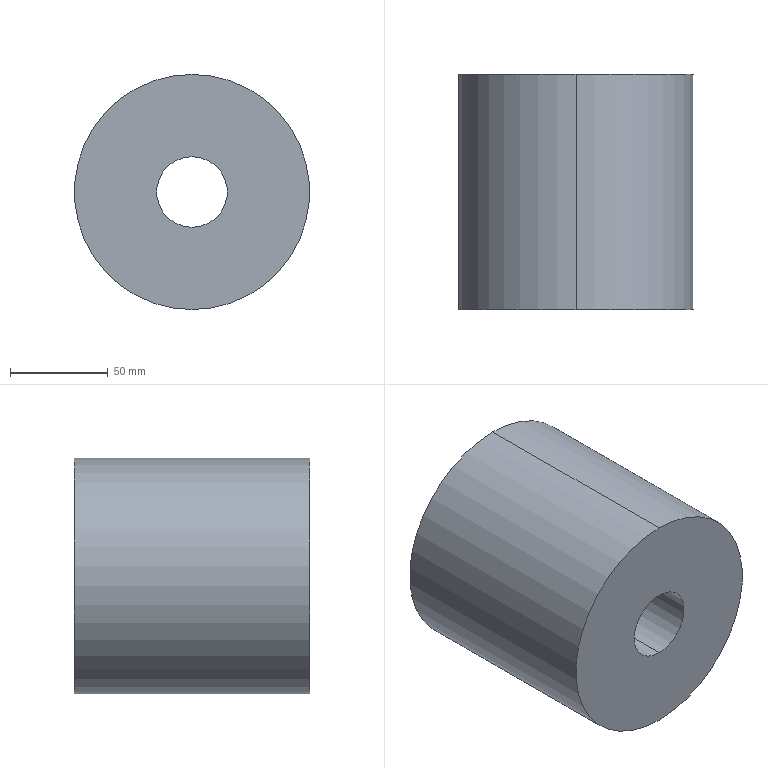Part | STEP file | 1 solid | 6 faces | box 120 x 120 x 120 mm | volume 1235023 mm3 | cylinder 4 | plane 2 | commonest cylinder face diameters 36 x2 120 x2
STEP:
#1=CARTESIAN_POINT('',(0.,0.,0.));
#2=DIRECTION('',(0.,0.,1.));
#3=DIRECTION('',(1.,0.,0.));
#4=AXIS2_PLACEMENT_3D('',#1,#2,#3);
#5=CARTESIAN_POINT('',(0.,60.,-18.));
#6=VERTEX_POINT('',#5);
#7=CARTESIAN_POINT('',(0.,-60.,-18.));
#8=VERTEX_POINT('',#7);
#9=CARTESIAN_POINT('',(0.,60.,-18.));
#10=DIRECTION('',(0.,-1.,0.));
#11=VECTOR('',#10,1.);
#12=LINE('',#9,#11);
#13=CARTESIAN_POINT('',(0.,60.,0.));
#14=DIRECTION('',(0.,-1.,0.));
#15=DIRECTION('',(0.,0.,-1.));
#16=AXIS2_PLACEMENT_3D('',#13,#14,#15);
#17=CYLINDRICAL_SURFACE('',#16,18.);
#18=CARTESIAN_POINT('',(6.283,0.));
#19=DIRECTION('',(0.,1.));
#20=VECTOR('',#19,1.);
#21=LINE('',#18,#20);
#22=(GEOMETRIC_REPRESENTATION_CONTEXT(2)PARAMETRIC_REPRESENTATION_CONTEXT()REPRESENTATION_CONTEXT('',''));
#23=DEFINITIONAL_REPRESENTATION('',(#21),#22);
#24=PCURVE('',#17,#23);
#25=CARTESIAN_POINT('',(0.,60.,0.));
#26=DIRECTION('',(0.,-1.,0.));
#27=DIRECTION('',(0.,0.,-1.));
#28=AXIS2_PLACEMENT_3D('',#25,#26,#27);
#29=CYLINDRICAL_SURFACE('',#28,18.);
#30=CARTESIAN_POINT('',(0.,0.));
#31=DIRECTION('',(0.,1.));
#32=VECTOR('',#31,1.);
#33=LINE('',#30,#32);
#34=(GEOMETRIC_REPRESENTATION_CONTEXT(2)PARAMETRIC_REPRESENTATION_CONTEXT()REPRESENTATION_CONTEXT('',''));
#35=DEFINITIONAL_REPRESENTATION('',(#33),#34);
#36=PCURVE('',#29,#35);
#37=SURFACE_CURVE('',#12,(#24,#36),.PCURVE_S1.);
#38=EDGE_CURVE('',#6,#8,#37,.T.);
#39=ORIENTED_EDGE('',*,*,#38,.T.);
#40=CARTESIAN_POINT('',(0.,-60.,18.));
#41=VERTEX_POINT('',#40);
#42=CARTESIAN_POINT('',(0.,-60.,0.));
#43=DIRECTION('',(0.,1.,0.));
#44=DIRECTION('',(0.,0.,1.));
#45=AXIS2_PLACEMENT_3D('',#42,#43,#44);
#46=CIRCLE('',#45,18.);
#47=CARTESIAN_POINT('',(9.425,120.));
#48=DIRECTION('',(-1.,0.));
#49=VECTOR('',#48,1.);
#50=LINE('',#47,#49);
#51=(GEOMETRIC_REPRESENTATION_CONTEXT(2)PARAMETRIC_REPRESENTATION_CONTEXT()REPRESENTATION_CONTEXT('',''));
#52=DEFINITIONAL_REPRESENTATION('',(#50),#51);
#53=PCURVE('',#17,#52);
#54=CARTESIAN_POINT('',(0.,-60.,0.));
#55=DIRECTION('',(0.,1.,0.));
#56=DIRECTION('',(0.,0.,1.));
#57=AXIS2_PLACEMENT_3D('',#54,#55,#56);
#58=PLANE('',#57);
#59=CARTESIAN_POINT('',(0.,0.));
#60=DIRECTION('',(1.,0.));
#61=AXIS2_PLACEMENT_2D('',#59,#60);
#62=CIRCLE('',#61,18.);
#63=(GEOMETRIC_REPRESENTATION_CONTEXT(2)PARAMETRIC_REPRESENTATION_CONTEXT()REPRESENTATION_CONTEXT('',''));
#64=DEFINITIONAL_REPRESENTATION('',(#62),#63);
#65=PCURVE('',#58,#64);
#66=SURFACE_CURVE('',#46,(#53,#65),.PCURVE_S1.);
#67=EDGE_CURVE('',#8,#41,#66,.T.);
#68=ORIENTED_EDGE('',*,*,#67,.T.);
#69=CARTESIAN_POINT('',(0.,60.,18.));
#70=VERTEX_POINT('',#69);
#71=CARTESIAN_POINT('',(0.,60.,18.));
#72=DIRECTION('',(0.,-1.,0.));
#73=VECTOR('',#72,1.);
#74=LINE('',#71,#73);
#75=CARTESIAN_POINT('',(3.142,0.));
#76=DIRECTION('',(0.,1.));
#77=VECTOR('',#76,1.);
#78=LINE('',#75,#77);
#79=(GEOMETRIC_REPRESENTATION_CONTEXT(2)PARAMETRIC_REPRESENTATION_CONTEXT()REPRESENTATION_CONTEXT('',''));
#80=DEFINITIONAL_REPRESENTATION('',(#78),#79);
#81=PCURVE('',#17,#80);
#82=CARTESIAN_POINT('',(3.142,0.));
#83=DIRECTION('',(0.,1.));
#84=VECTOR('',#83,1.);
#85=LINE('',#82,#84);
#86=(GEOMETRIC_REPRESENTATION_CONTEXT(2)PARAMETRIC_REPRESENTATION_CONTEXT()REPRESENTATION_CONTEXT('',''));
#87=DEFINITIONAL_REPRESENTATION('',(#85),#86);
#88=PCURVE('',#29,#87);
#89=SURFACE_CURVE('',#74,(#81,#88),.PCURVE_S1.);
#90=EDGE_CURVE('',#70,#41,#89,.T.);
#91=ORIENTED_EDGE('',*,*,#90,.F.);
#92=CARTESIAN_POINT('',(0.,60.,0.));
#93=DIRECTION('',(0.,1.,0.));
#94=DIRECTION('',(0.,0.,1.));
#95=AXIS2_PLACEMENT_3D('',#92,#93,#94);
#96=CIRCLE('',#95,18.);
#97=CARTESIAN_POINT('',(9.425,0.));
#98=DIRECTION('',(-1.,0.));
#99=VECTOR('',#98,1.);
#100=LINE('',#97,#99);
#101=(GEOMETRIC_REPRESENTATION_CONTEXT(2)PARAMETRIC_REPRESENTATION_CONTEXT()REPRESENTATION_CONTEXT('',''));
#102=DEFINITIONAL_REPRESENTATION('',(#100),#101);
#103=PCURVE('',#17,#102);
#104=CARTESIAN_POINT('',(0.,60.,0.));
#105=DIRECTION('',(0.,1.,0.));
#106=DIRECTION('',(0.,0.,1.));
#107=AXIS2_PLACEMENT_3D('',#104,#105,#106);
#108=PLANE('',#107);
#109=CARTESIAN_POINT('',(0.,0.));
#110=DIRECTION('',(1.,0.));
#111=AXIS2_PLACEMENT_2D('',#109,#110);
#112=CIRCLE('',#111,18.);
#113=(GEOMETRIC_REPRESENTATION_CONTEXT(2)PARAMETRIC_REPRESENTATION_CONTEXT()REPRESENTATION_CONTEXT('',''));
#114=DEFINITIONAL_REPRESENTATION('',(#112),#113);
#115=PCURVE('',#108,#114);
#116=SURFACE_CURVE('',#96,(#103,#115),.PCURVE_S1.);
#117=EDGE_CURVE('',#6,#70,#116,.T.);
#118=ORIENTED_EDGE('',*,*,#117,.F.);
#119=EDGE_LOOP('',(#39,#68,#91,#118));
#120=FACE_BOUND('',#119,.F.);
#121=ADVANCED_FACE('',(#120),#17,.F.);
#122=CARTESIAN_POINT('',(0.,60.,60.));
#123=VERTEX_POINT('',#122);
#124=CARTESIAN_POINT('',(0.,60.,-60.));
#125=VERTEX_POINT('',#124);
#126=CARTESIAN_POINT('',(0.,60.,0.));
#127=DIRECTION('',(0.,1.,0.));
#128=DIRECTION('',(0.,0.,1.));
#129=AXIS2_PLACEMENT_3D('',#126,#127,#128);
#130=CIRCLE('',#129,60.);
#131=CARTESIAN_POINT('',(0.,60.,0.));
#132=DIRECTION('',(0.,-1.,0.));
#133=DIRECTION('',(0.,0.,-1.));
#134=AXIS2_PLACEMENT_3D('',#131,#132,#133);
#135=CYLINDRICAL_SURFACE('',#134,60.);
#136=CARTESIAN_POINT('',(3.142,0.));
#137=DIRECTION('',(-1.,0.));
#138=VECTOR('',#137,1.);
#139=LINE('',#136,#138);
#140=(GEOMETRIC_REPRESENTATION_CONTEXT(2)PARAMETRIC_REPRESENTATION_CONTEXT()REPRESENTATION_CONTEXT('',''));
#141=DEFINITIONAL_REPRESENTATION('',(#139),#140);
#142=PCURVE('',#135,#141);
#143=CARTESIAN_POINT('',(0.,0.));
#144=DIRECTION('',(1.,0.));
#145=AXIS2_PLACEMENT_2D('',#143,#144);
#146=CIRCLE('',#145,60.);
#147=(GEOMETRIC_REPRESENTATION_CONTEXT(2)PARAMETRIC_REPRESENTATION_CONTEXT()REPRESENTATION_CONTEXT('',''));
#148=DEFINITIONAL_REPRESENTATION('',(#146),#147);
#149=PCURVE('',#108,#148);
#150=SURFACE_CURVE('',#130,(#142,#149),.PCURVE_S1.);
#151=EDGE_CURVE('',#123,#125,#150,.T.);
#152=ORIENTED_EDGE('',*,*,#151,.F.);
#153=CARTESIAN_POINT('',(0.,-60.,60.));
#154=VERTEX_POINT('',#153);
#155=CARTESIAN_POINT('',(0.,60.,60.));
#156=DIRECTION('',(0.,-1.,0.));
#157=VECTOR('',#156,1.);
#158=LINE('',#155,#157);
#159=CARTESIAN_POINT('',(3.142,0.));
#160=DIRECTION('',(0.,1.));
#161=VECTOR('',#160,1.);
#162=LINE('',#159,#161);
#163=(GEOMETRIC_REPRESENTATION_CONTEXT(2)PARAMETRIC_REPRESENTATION_CONTEXT()REPRESENTATION_CONTEXT('',''));
#164=DEFINITIONAL_REPRESENTATION('',(#162),#163);
#165=PCURVE('',#135,#164);
#166=CARTESIAN_POINT('',(0.,60.,0.));
#167=DIRECTION('',(0.,-1.,0.));
#168=DIRECTION('',(0.,0.,-1.));
#169=AXIS2_PLACEMENT_3D('',#166,#167,#168);
#170=CYLINDRICAL_SURFACE('',#169,60.);
#171=CARTESIAN_POINT('',(3.142,0.));
#172=DIRECTION('',(0.,1.));
#173=VECTOR('',#172,1.);
#174=LINE('',#171,#173);
#175=(GEOMETRIC_REPRESENTATION_CONTEXT(2)PARAMETRIC_REPRESENTATION_CONTEXT()REPRESENTATION_CONTEXT('',''));
#176=DEFINITIONAL_REPRESENTATION('',(#174),#175);
#177=PCURVE('',#170,#176);
#178=SURFACE_CURVE('',#158,(#165,#177),.PCURVE_S1.);
#179=EDGE_CURVE('',#123,#154,#178,.T.);
#180=ORIENTED_EDGE('',*,*,#179,.T.);
#181=CARTESIAN_POINT('',(0.,-60.,-60.));
#182=VERTEX_POINT('',#181);
#183=CARTESIAN_POINT('',(0.,-60.,0.));
#184=DIRECTION('',(0.,1.,0.));
#185=DIRECTION('',(0.,0.,1.));
#186=AXIS2_PLACEMENT_3D('',#183,#184,#185);
#187=CIRCLE('',#186,60.);
#188=CARTESIAN_POINT('',(3.142,120.));
#189=DIRECTION('',(-1.,0.));
#190=VECTOR('',#189,1.);
#191=LINE('',#188,#190);
#192=(GEOMETRIC_REPRESENTATION_CONTEXT(2)PARAMETRIC_REPRESENTATION_CONTEXT()REPRESENTATION_CONTEXT('',''));
#193=DEFINITIONAL_REPRESENTATION('',(#191),#192);
#194=PCURVE('',#135,#193);
#195=CARTESIAN_POINT('',(0.,0.));
#196=DIRECTION('',(1.,0.));
#197=AXIS2_PLACEMENT_2D('',#195,#196);
#198=CIRCLE('',#197,60.);
#199=(GEOMETRIC_REPRESENTATION_CONTEXT(2)PARAMETRIC_REPRESENTATION_CONTEXT()REPRESENTATION_CONTEXT('',''));
#200=DEFINITIONAL_REPRESENTATION('',(#198),#199);
#201=PCURVE('',#58,#200);
#202=SURFACE_CURVE('',#187,(#194,#201),.PCURVE_S1.);
#203=EDGE_CURVE('',#154,#182,#202,.T.);
#204=ORIENTED_EDGE('',*,*,#203,.T.);
#205=CARTESIAN_POINT('',(0.,60.,-60.));
#206=DIRECTION('',(0.,-1.,0.));
#207=VECTOR('',#206,1.);
#208=LINE('',#205,#207);
#209=CARTESIAN_POINT('',(0.,0.));
#210=DIRECTION('',(0.,1.));
#211=VECTOR('',#210,1.);
#212=LINE('',#209,#211);
#213=(GEOMETRIC_REPRESENTATION_CONTEXT(2)PARAMETRIC_REPRESENTATION_CONTEXT()REPRESENTATION_CONTEXT('',''));
#214=DEFINITIONAL_REPRESENTATION('',(#212),#213);
#215=PCURVE('',#135,#214);
#216=CARTESIAN_POINT('',(6.283,0.));
#217=DIRECTION('',(0.,1.));
#218=VECTOR('',#217,1.);
#219=LINE('',#216,#218);
#220=(GEOMETRIC_REPRESENTATION_CONTEXT(2)PARAMETRIC_REPRESENTATION_CONTEXT()REPRESENTATION_CONTEXT('',''));
#221=DEFINITIONAL_REPRESENTATION('',(#219),#220);
#222=PCURVE('',#170,#221);
#223=SURFACE_CURVE('',#208,(#215,#222),.PCURVE_S1.);
#224=EDGE_CURVE('',#125,#182,#223,.T.);
#225=ORIENTED_EDGE('',*,*,#224,.F.);
#226=EDGE_LOOP('',(#152,#180,#204,#225));
#227=FACE_BOUND('',#226,.T.);
#228=ADVANCED_FACE('',(#227),#135,.T.);
#229=CARTESIAN_POINT('',(0.,60.,0.));
#230=DIRECTION('',(0.,1.,0.));
#231=DIRECTION('',(0.,0.,1.));
#232=AXIS2_PLACEMENT_3D('',#229,#230,#231);
#233=CIRCLE('',#232,60.);
#234=CARTESIAN_POINT('',(0.,0.));
#235=DIRECTION('',(1.,0.));
#236=AXIS2_PLACEMENT_2D('',#234,#235);
#237=CIRCLE('',#236,60.);
#238=(GEOMETRIC_REPRESENTATION_CONTEXT(2)PARAMETRIC_REPRESENTATION_CONTEXT()REPRESENTATION_CONTEXT('',''));
#239=DEFINITIONAL_REPRESENTATION('',(#237),#238);
#240=PCURVE('',#108,#239);
#241=CARTESIAN_POINT('',(9.425,0.));
#242=DIRECTION('',(-1.,0.));
#243=VECTOR('',#242,1.);
#244=LINE('',#241,#243);
#245=(GEOMETRIC_REPRESENTATION_CONTEXT(2)PARAMETRIC_REPRESENTATION_CONTEXT()REPRESENTATION_CONTEXT('',''));
#246=DEFINITIONAL_REPRESENTATION('',(#244),#245);
#247=PCURVE('',#170,#246);
#248=SURFACE_CURVE('',#233,(#240,#247),.PCURVE_S1.);
#249=EDGE_CURVE('',#125,#123,#248,.T.);
#250=ORIENTED_EDGE('',*,*,#249,.T.);
#251=ORIENTED_EDGE('',*,*,#151,.T.);
#252=EDGE_LOOP('',(#250,#251));
#253=FACE_BOUND('',#252,.T.);
#254=ORIENTED_EDGE('',*,*,#117,.F.);
#255=CARTESIAN_POINT('',(0.,60.,0.));
#256=DIRECTION('',(0.,1.,0.));
#257=DIRECTION('',(0.,0.,1.));
#258=AXIS2_PLACEMENT_3D('',#255,#256,#257);
#259=CIRCLE('',#258,18.);
#260=CARTESIAN_POINT('',(0.,0.));
#261=DIRECTION('',(1.,0.));
#262=AXIS2_PLACEMENT_2D('',#260,#261);
#263=CIRCLE('',#262,18.);
#264=(GEOMETRIC_REPRESENTATION_CONTEXT(2)PARAMETRIC_REPRESENTATION_CONTEXT()REPRESENTATION_CONTEXT('',''));
#265=DEFINITIONAL_REPRESENTATION('',(#263),#264);
#266=PCURVE('',#108,#265);
#267=CARTESIAN_POINT('',(3.142,0.));
#268=DIRECTION('',(-1.,0.));
#269=VECTOR('',#268,1.);
#270=LINE('',#267,#269);
#271=(GEOMETRIC_REPRESENTATION_CONTEXT(2)PARAMETRIC_REPRESENTATION_CONTEXT()REPRESENTATION_CONTEXT('',''));
#272=DEFINITIONAL_REPRESENTATION('',(#270),#271);
#273=PCURVE('',#29,#272);
#274=SURFACE_CURVE('',#259,(#266,#273),.PCURVE_S1.);
#275=EDGE_CURVE('',#70,#6,#274,.T.);
#276=ORIENTED_EDGE('',*,*,#275,.F.);
#277=EDGE_LOOP('',(#254,#276));
#278=FACE_BOUND('',#277,.T.);
#279=ADVANCED_FACE('',(#253,#278),#108,.T.);
#280=CARTESIAN_POINT('',(0.,-60.,0.));
#281=DIRECTION('',(0.,1.,0.));
#282=DIRECTION('',(0.,0.,1.));
#283=AXIS2_PLACEMENT_3D('',#280,#281,#282);
#284=CIRCLE('',#283,60.);
#285=CARTESIAN_POINT('',(0.,0.));
#286=DIRECTION('',(1.,0.));
#287=AXIS2_PLACEMENT_2D('',#285,#286);
#288=CIRCLE('',#287,60.);
#289=(GEOMETRIC_REPRESENTATION_CONTEXT(2)PARAMETRIC_REPRESENTATION_CONTEXT()REPRESENTATION_CONTEXT('',''));
#290=DEFINITIONAL_REPRESENTATION('',(#288),#289);
#291=PCURVE('',#58,#290);
#292=CARTESIAN_POINT('',(9.425,120.));
#293=DIRECTION('',(-1.,0.));
#294=VECTOR('',#293,1.);
#295=LINE('',#292,#294);
#296=(GEOMETRIC_REPRESENTATION_CONTEXT(2)PARAMETRIC_REPRESENTATION_CONTEXT()REPRESENTATION_CONTEXT('',''));
#297=DEFINITIONAL_REPRESENTATION('',(#295),#296);
#298=PCURVE('',#170,#297);
#299=SURFACE_CURVE('',#284,(#291,#298),.PCURVE_S1.);
#300=EDGE_CURVE('',#182,#154,#299,.T.);
#301=ORIENTED_EDGE('',*,*,#300,.F.);
#302=ORIENTED_EDGE('',*,*,#203,.F.);
#303=EDGE_LOOP('',(#301,#302));
#304=FACE_BOUND('',#303,.T.);
#305=ORIENTED_EDGE('',*,*,#67,.T.);
#306=CARTESIAN_POINT('',(0.,-60.,0.));
#307=DIRECTION('',(0.,1.,0.));
#308=DIRECTION('',(0.,0.,1.));
#309=AXIS2_PLACEMENT_3D('',#306,#307,#308);
#310=CIRCLE('',#309,18.);
#311=CARTESIAN_POINT('',(0.,0.));
#312=DIRECTION('',(1.,0.));
#313=AXIS2_PLACEMENT_2D('',#311,#312);
#314=CIRCLE('',#313,18.);
#315=(GEOMETRIC_REPRESENTATION_CONTEXT(2)PARAMETRIC_REPRESENTATION_CONTEXT()REPRESENTATION_CONTEXT('',''));
#316=DEFINITIONAL_REPRESENTATION('',(#314),#315);
#317=PCURVE('',#58,#316);
#318=CARTESIAN_POINT('',(3.142,120.));
#319=DIRECTION('',(-1.,0.));
#320=VECTOR('',#319,1.);
#321=LINE('',#318,#320);
#322=(GEOMETRIC_REPRESENTATION_CONTEXT(2)PARAMETRIC_REPRESENTATION_CONTEXT()REPRESENTATION_CONTEXT('',''));
#323=DEFINITIONAL_REPRESENTATION('',(#321),#322);
#324=PCURVE('',#29,#323);
#325=SURFACE_CURVE('',#310,(#317,#324),.PCURVE_S1.);
#326=EDGE_CURVE('',#41,#8,#325,.T.);
#327=ORIENTED_EDGE('',*,*,#326,.T.);
#328=EDGE_LOOP('',(#305,#327));
#329=FACE_BOUND('',#328,.T.);
#330=ADVANCED_FACE('',(#304,#329),#58,.F.);
#331=ORIENTED_EDGE('',*,*,#179,.F.);
#332=ORIENTED_EDGE('',*,*,#249,.F.);
#333=ORIENTED_EDGE('',*,*,#224,.T.);
#334=ORIENTED_EDGE('',*,*,#300,.T.);
#335=EDGE_LOOP('',(#331,#332,#333,#334));
#336=FACE_BOUND('',#335,.T.);
#337=ADVANCED_FACE('',(#336),#170,.T.);
#338=ORIENTED_EDGE('',*,*,#326,.T.);
#339=ORIENTED_EDGE('',*,*,#38,.F.);
#340=ORIENTED_EDGE('',*,*,#275,.F.);
#341=ORIENTED_EDGE('',*,*,#90,.T.);
#342=EDGE_LOOP('',(#338,#339,#340,#341));
#343=FACE_BOUND('',#342,.F.);
#344=ADVANCED_FACE('',(#343),#29,.F.);
#345=CLOSED_SHELL('',(#121,#228,#279,#330,#337,#344));
#346=MANIFOLD_SOLID_BREP('',#345);
#347=(LENGTH_UNIT()NAMED_UNIT(*)SI_UNIT(.MILLI.,.METRE.));
#348=UNCERTAINTY_MEASURE_WITH_UNIT(LENGTH_MEASURE(0.0000001),#347,'','');
#349=(NAMED_UNIT(*)PLANE_ANGLE_UNIT()SI_UNIT($,.RADIAN.));
#350=(NAMED_UNIT(*)SI_UNIT($,.STERADIAN.)SOLID_ANGLE_UNIT());
#351=(GEOMETRIC_REPRESENTATION_CONTEXT(3)GLOBAL_UNCERTAINTY_ASSIGNED_CONTEXT((#348))GLOBAL_UNIT_ASSIGNED_CONTEXT((#347,#349,#350))REPRESENTATION_CONTEXT('',''));
#352=ADVANCED_BREP_SHAPE_REPRESENTATION('',(#4,#346),#351);